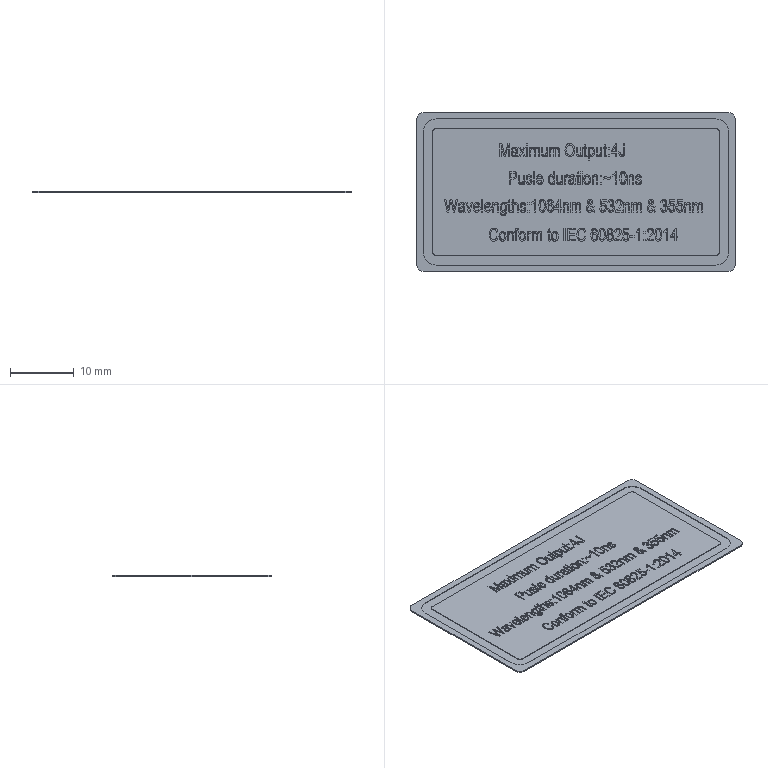Part | STEP file | IEC-MINGPAI.stp.STEP | 1 solid | 1896 faces | box 50 x 25 x 0.2 mm | volume 223.264 mm3 | spline 1188 | plane 696 | cylinder 12 | commonest cylinder face diameters 1 x4 2 x4 4 x4